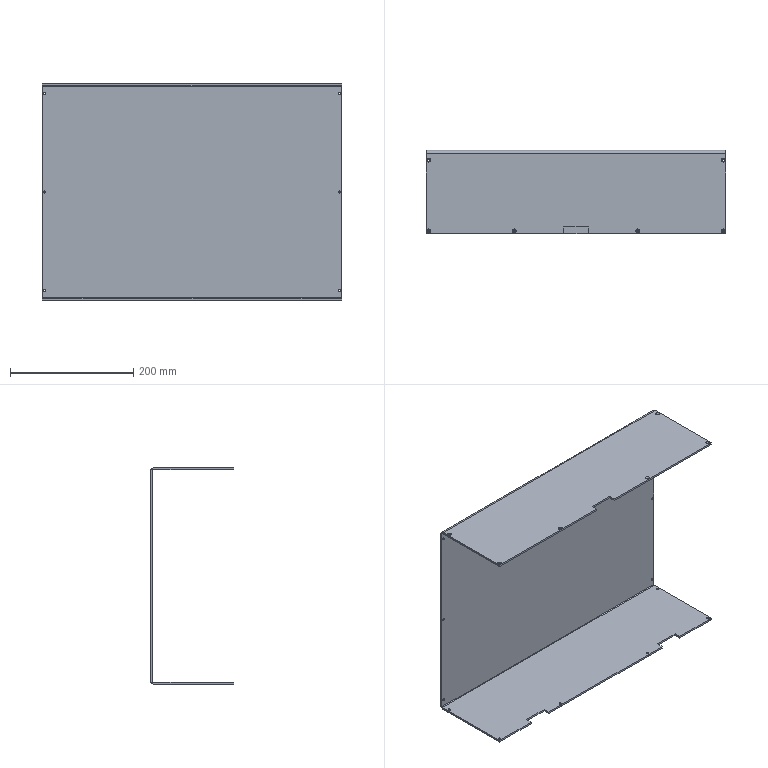Part | SolidWorks | features HoleWzd 3, Cut 2, Fillet 2, ICE 2, Extrusion 1 | 1 solid | 98 faces | box 485.5 x 135 x 351 mm | volume 883861 mm3 | cylinder 40 | cone 36 | plane 22 | commonest cylinder face diameters 3.4 x36 2 x2 12 x2